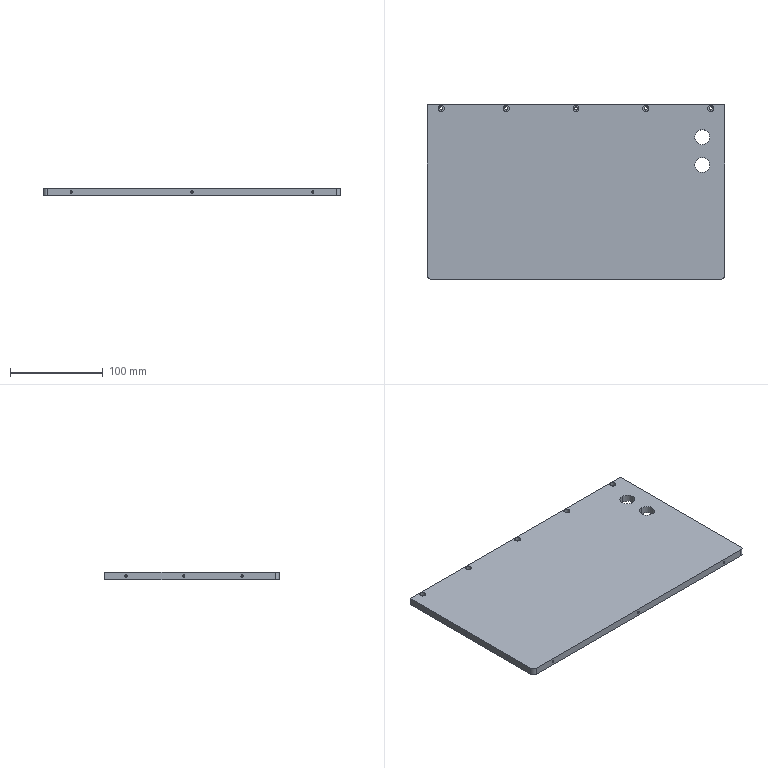Part | 1 solid | 73 faces | box 320 x 188 x 8 mm | volume 476820 mm3 | cylinder 44 | cone 18 | plane 11 | commonest cylinder face diameters 2.5 x18 3.4 x10 6.5 x10 16 x4 8 x2